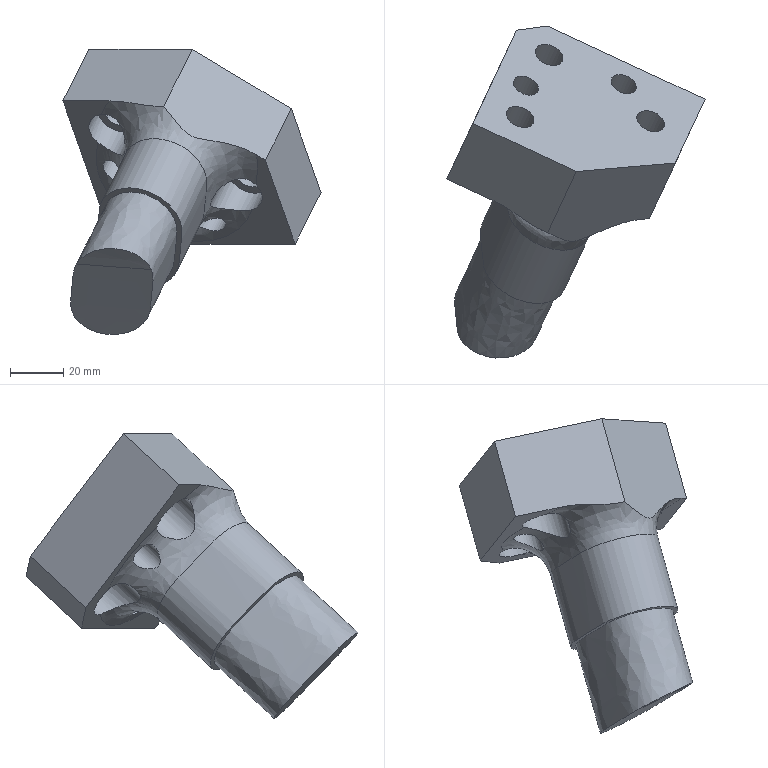Part | NX | features solid 2 | 1 solid | 25 faces | box 96.701 x 124.413 x 106.832 mm | volume 224536 mm3 | plane 12 | cylinder 8 | spline 5 | commonest cylinder face diameters 11 x3 17 x3 10 x2